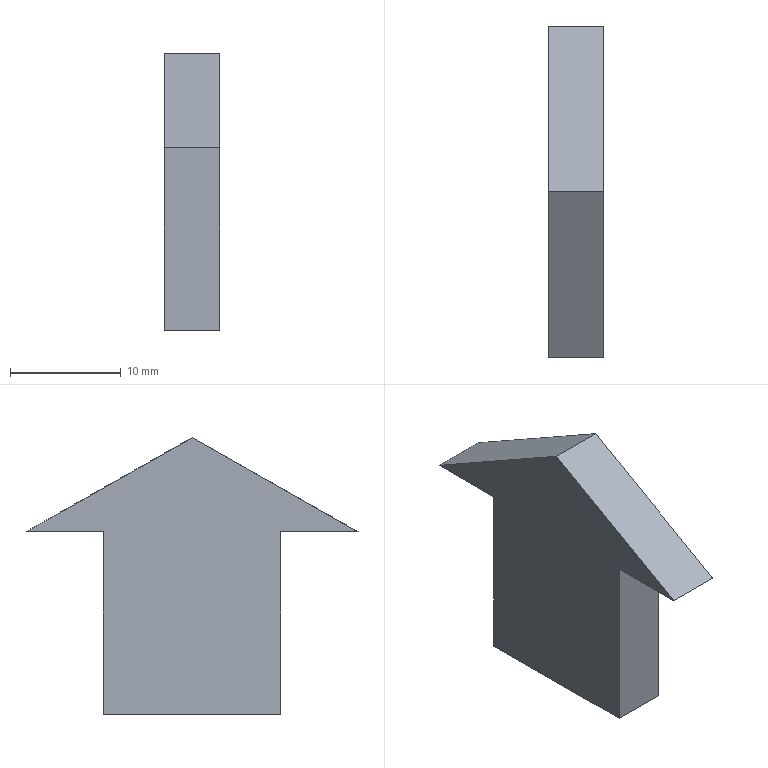Part | STEP file | 2_2_1-- | 1 solid | 9 faces | box 5 x 30 x 25 mm | volume 1957 mm3 | plane 9
STEP:
#1=CARTESIAN_POINT('',(0.,0.,0.));
#2=DIRECTION('',(0.,0.,1.));
#3=DIRECTION('',(1.,0.,0.));
#4=AXIS2_PLACEMENT_3D('',#1,#2,#3);
#5=CARTESIAN_POINT('',(-2.5,0.,50.));
#6=VERTEX_POINT('',#5);
#7=CARTESIAN_POINT('',(-2.5,-15.,41.5));
#8=VERTEX_POINT('',#7);
#9=CARTESIAN_POINT('',(-2.5,0.,50.));
#10=DIRECTION('',(0.,-0.87,-0.493));
#11=VECTOR('',#10,1.);
#12=LINE('',#9,#11);
#13=CARTESIAN_POINT('',(-2.5,0.,50.));
#14=DIRECTION('',(1.,0.,0.));
#15=DIRECTION('',(0.,0.,-1.));
#16=AXIS2_PLACEMENT_3D('',#13,#14,#15);
#17=PLANE('',#16);
#18=CARTESIAN_POINT('',(0.,0.));
#19=DIRECTION('',(0.493,-0.87));
#20=VECTOR('',#19,1.);
#21=LINE('',#18,#20);
#22=(GEOMETRIC_REPRESENTATION_CONTEXT(2)PARAMETRIC_REPRESENTATION_CONTEXT()REPRESENTATION_CONTEXT('',''));
#23=DEFINITIONAL_REPRESENTATION('',(#21),#22);
#24=PCURVE('',#17,#23);
#25=CARTESIAN_POINT('',(2.5,0.,50.));
#26=DIRECTION('',(0.,-0.493,0.87));
#27=DIRECTION('',(0.,-0.87,-0.493));
#28=AXIS2_PLACEMENT_3D('',#25,#26,#27);
#29=PLANE('',#28);
#30=CARTESIAN_POINT('',(0.,-5.));
#31=DIRECTION('',(1.,0.));
#32=VECTOR('',#31,1.);
#33=LINE('',#30,#32);
#34=(GEOMETRIC_REPRESENTATION_CONTEXT(2)PARAMETRIC_REPRESENTATION_CONTEXT()REPRESENTATION_CONTEXT('',''));
#35=DEFINITIONAL_REPRESENTATION('',(#33),#34);
#36=PCURVE('',#29,#35);
#37=SURFACE_CURVE('',#12,(#24,#36),.PCURVE_S1.);
#38=EDGE_CURVE('',#6,#8,#37,.T.);
#39=ORIENTED_EDGE('',*,*,#38,.F.);
#40=CARTESIAN_POINT('',(-2.5,15.,41.5));
#41=VERTEX_POINT('',#40);
#42=CARTESIAN_POINT('',(-2.5,15.,41.5));
#43=DIRECTION('',(0.,-0.87,0.493));
#44=VECTOR('',#43,1.);
#45=LINE('',#42,#44);
#46=CARTESIAN_POINT('',(8.5,15.));
#47=DIRECTION('',(-0.493,-0.87));
#48=VECTOR('',#47,1.);
#49=LINE('',#46,#48);
#50=(GEOMETRIC_REPRESENTATION_CONTEXT(2)PARAMETRIC_REPRESENTATION_CONTEXT()REPRESENTATION_CONTEXT('',''));
#51=DEFINITIONAL_REPRESENTATION('',(#49),#50);
#52=PCURVE('',#17,#51);
#53=CARTESIAN_POINT('',(2.5,15.,41.5));
#54=DIRECTION('',(0.,0.493,0.87));
#55=DIRECTION('',(0.,-0.87,0.493));
#56=AXIS2_PLACEMENT_3D('',#53,#54,#55);
#57=PLANE('',#56);
#58=CARTESIAN_POINT('',(0.,-5.));
#59=DIRECTION('',(1.,0.));
#60=VECTOR('',#59,1.);
#61=LINE('',#58,#60);
#62=(GEOMETRIC_REPRESENTATION_CONTEXT(2)PARAMETRIC_REPRESENTATION_CONTEXT()REPRESENTATION_CONTEXT('',''));
#63=DEFINITIONAL_REPRESENTATION('',(#61),#62);
#64=PCURVE('',#57,#63);
#65=SURFACE_CURVE('',#45,(#52,#64),.PCURVE_S1.);
#66=EDGE_CURVE('',#41,#6,#65,.T.);
#67=ORIENTED_EDGE('',*,*,#66,.F.);
#68=CARTESIAN_POINT('',(-2.5,8.,41.5));
#69=VERTEX_POINT('',#68);
#70=CARTESIAN_POINT('',(-2.5,0.,41.5));
#71=DIRECTION('',(0.,1.,0.));
#72=VECTOR('',#71,1.);
#73=LINE('',#70,#72);
#74=CARTESIAN_POINT('',(8.5,0.));
#75=DIRECTION('',(0.,1.));
#76=VECTOR('',#75,1.);
#77=LINE('',#74,#76);
#78=(GEOMETRIC_REPRESENTATION_CONTEXT(2)PARAMETRIC_REPRESENTATION_CONTEXT()REPRESENTATION_CONTEXT('',''));
#79=DEFINITIONAL_REPRESENTATION('',(#77),#78);
#80=PCURVE('',#17,#79);
#81=CARTESIAN_POINT('',(2.5,8.,41.5));
#82=DIRECTION('',(0.,0.,-1.));
#83=DIRECTION('',(-1.,0.,0.));
#84=AXIS2_PLACEMENT_3D('',#81,#82,#83);
#85=PLANE('',#84);
#86=CARTESIAN_POINT('',(5.,-8.));
#87=DIRECTION('',(0.,1.));
#88=VECTOR('',#87,1.);
#89=LINE('',#86,#88);
#90=(GEOMETRIC_REPRESENTATION_CONTEXT(2)PARAMETRIC_REPRESENTATION_CONTEXT()REPRESENTATION_CONTEXT('',''));
#91=DEFINITIONAL_REPRESENTATION('',(#89),#90);
#92=PCURVE('',#85,#91);
#93=SURFACE_CURVE('',#73,(#80,#92),.PCURVE_S1.);
#94=EDGE_CURVE('',#69,#41,#93,.T.);
#95=ORIENTED_EDGE('',*,*,#94,.F.);
#96=CARTESIAN_POINT('',(-2.5,8.,25.));
#97=VERTEX_POINT('',#96);
#98=CARTESIAN_POINT('',(-2.5,8.,50.));
#99=DIRECTION('',(0.,0.,1.));
#100=VECTOR('',#99,1.);
#101=LINE('',#98,#100);
#102=CARTESIAN_POINT('',(0.,8.));
#103=DIRECTION('',(-1.,0.));
#104=VECTOR('',#103,1.);
#105=LINE('',#102,#104);
#106=(GEOMETRIC_REPRESENTATION_CONTEXT(2)PARAMETRIC_REPRESENTATION_CONTEXT()REPRESENTATION_CONTEXT('',''));
#107=DEFINITIONAL_REPRESENTATION('',(#105),#106);
#108=PCURVE('',#17,#107);
#109=CARTESIAN_POINT('',(2.5,8.,25.));
#110=DIRECTION('',(0.,1.,0.));
#111=DIRECTION('',(0.,0.,1.));
#112=AXIS2_PLACEMENT_3D('',#109,#110,#111);
#113=PLANE('',#112);
#114=CARTESIAN_POINT('',(25.,-5.));
#115=DIRECTION('',(1.,0.));
#116=VECTOR('',#115,1.);
#117=LINE('',#114,#116);
#118=(GEOMETRIC_REPRESENTATION_CONTEXT(2)PARAMETRIC_REPRESENTATION_CONTEXT()REPRESENTATION_CONTEXT('',''));
#119=DEFINITIONAL_REPRESENTATION('',(#117),#118);
#120=PCURVE('',#113,#119);
#121=SURFACE_CURVE('',#101,(#108,#120),.PCURVE_S1.);
#122=EDGE_CURVE('',#97,#69,#121,.T.);
#123=ORIENTED_EDGE('',*,*,#122,.F.);
#124=CARTESIAN_POINT('',(-2.5,-8.,25.));
#125=VERTEX_POINT('',#124);
#126=CARTESIAN_POINT('',(-2.5,0.,25.));
#127=DIRECTION('',(0.,1.,0.));
#128=VECTOR('',#127,1.);
#129=LINE('',#126,#128);
#130=CARTESIAN_POINT('',(25.,0.));
#131=DIRECTION('',(0.,1.));
#132=VECTOR('',#131,1.);
#133=LINE('',#130,#132);
#134=(GEOMETRIC_REPRESENTATION_CONTEXT(2)PARAMETRIC_REPRESENTATION_CONTEXT()REPRESENTATION_CONTEXT('',''));
#135=DEFINITIONAL_REPRESENTATION('',(#133),#134);
#136=PCURVE('',#17,#135);
#137=CARTESIAN_POINT('',(2.5,-8.,25.));
#138=DIRECTION('',(0.,0.,-1.));
#139=DIRECTION('',(-1.,0.,0.));
#140=AXIS2_PLACEMENT_3D('',#137,#138,#139);
#141=PLANE('',#140);
#142=CARTESIAN_POINT('',(5.,8.));
#143=DIRECTION('',(0.,1.));
#144=VECTOR('',#143,1.);
#145=LINE('',#142,#144);
#146=(GEOMETRIC_REPRESENTATION_CONTEXT(2)PARAMETRIC_REPRESENTATION_CONTEXT()REPRESENTATION_CONTEXT('',''));
#147=DEFINITIONAL_REPRESENTATION('',(#145),#146);
#148=PCURVE('',#141,#147);
#149=SURFACE_CURVE('',#129,(#136,#148),.PCURVE_S1.);
#150=EDGE_CURVE('',#125,#97,#149,.T.);
#151=ORIENTED_EDGE('',*,*,#150,.F.);
#152=CARTESIAN_POINT('',(-2.5,-8.,41.5));
#153=VERTEX_POINT('',#152);
#154=CARTESIAN_POINT('',(-2.5,-8.,50.));
#155=DIRECTION('',(0.,0.,-1.));
#156=VECTOR('',#155,1.);
#157=LINE('',#154,#156);
#158=CARTESIAN_POINT('',(0.,-8.));
#159=DIRECTION('',(1.,0.));
#160=VECTOR('',#159,1.);
#161=LINE('',#158,#160);
#162=(GEOMETRIC_REPRESENTATION_CONTEXT(2)PARAMETRIC_REPRESENTATION_CONTEXT()REPRESENTATION_CONTEXT('',''));
#163=DEFINITIONAL_REPRESENTATION('',(#161),#162);
#164=PCURVE('',#17,#163);
#165=CARTESIAN_POINT('',(2.5,-8.,41.5));
#166=DIRECTION('',(0.,-1.,0.));
#167=DIRECTION('',(0.,0.,-1.));
#168=AXIS2_PLACEMENT_3D('',#165,#166,#167);
#169=PLANE('',#168);
#170=CARTESIAN_POINT('',(-8.5,-5.));
#171=DIRECTION('',(1.,0.));
#172=VECTOR('',#171,1.);
#173=LINE('',#170,#172);
#174=(GEOMETRIC_REPRESENTATION_CONTEXT(2)PARAMETRIC_REPRESENTATION_CONTEXT()REPRESENTATION_CONTEXT('',''));
#175=DEFINITIONAL_REPRESENTATION('',(#173),#174);
#176=PCURVE('',#169,#175);
#177=SURFACE_CURVE('',#157,(#164,#176),.PCURVE_S1.);
#178=EDGE_CURVE('',#153,#125,#177,.T.);
#179=ORIENTED_EDGE('',*,*,#178,.F.);
#180=CARTESIAN_POINT('',(-2.5,0.,41.5));
#181=DIRECTION('',(0.,1.,0.));
#182=VECTOR('',#181,1.);
#183=LINE('',#180,#182);
#184=CARTESIAN_POINT('',(8.5,0.));
#185=DIRECTION('',(0.,1.));
#186=VECTOR('',#185,1.);
#187=LINE('',#184,#186);
#188=(GEOMETRIC_REPRESENTATION_CONTEXT(2)PARAMETRIC_REPRESENTATION_CONTEXT()REPRESENTATION_CONTEXT('',''));
#189=DEFINITIONAL_REPRESENTATION('',(#187),#188);
#190=PCURVE('',#17,#189);
#191=CARTESIAN_POINT('',(2.5,-15.,41.5));
#192=DIRECTION('',(0.,0.,-1.));
#193=DIRECTION('',(-1.,0.,0.));
#194=AXIS2_PLACEMENT_3D('',#191,#192,#193);
#195=PLANE('',#194);
#196=CARTESIAN_POINT('',(5.,15.));
#197=DIRECTION('',(0.,1.));
#198=VECTOR('',#197,1.);
#199=LINE('',#196,#198);
#200=(GEOMETRIC_REPRESENTATION_CONTEXT(2)PARAMETRIC_REPRESENTATION_CONTEXT()REPRESENTATION_CONTEXT('',''));
#201=DEFINITIONAL_REPRESENTATION('',(#199),#200);
#202=PCURVE('',#195,#201);
#203=SURFACE_CURVE('',#183,(#190,#202),.PCURVE_S1.);
#204=EDGE_CURVE('',#8,#153,#203,.T.);
#205=ORIENTED_EDGE('',*,*,#204,.F.);
#206=EDGE_LOOP('',(#39,#67,#95,#123,#151,#179,#205));
#207=FACE_BOUND('',#206,.T.);
#208=ADVANCED_FACE('',(#207),#17,.F.);
#209=CARTESIAN_POINT('',(2.5,-8.,41.5));
#210=VERTEX_POINT('',#209);
#211=CARTESIAN_POINT('',(2.5,-15.,41.5));
#212=VERTEX_POINT('',#211);
#213=CARTESIAN_POINT('',(2.5,-15.,41.5));
#214=DIRECTION('',(0.,-1.,0.));
#215=VECTOR('',#214,1.);
#216=LINE('',#213,#215);
#217=CARTESIAN_POINT('',(0.,0.));
#218=DIRECTION('',(0.,-1.));
#219=VECTOR('',#218,1.);
#220=LINE('',#217,#219);
#221=(GEOMETRIC_REPRESENTATION_CONTEXT(2)PARAMETRIC_REPRESENTATION_CONTEXT()REPRESENTATION_CONTEXT('',''));
#222=DEFINITIONAL_REPRESENTATION('',(#220),#221);
#223=PCURVE('',#195,#222);
#224=CARTESIAN_POINT('',(2.5,0.,50.));
#225=DIRECTION('',(1.,0.,0.));
#226=DIRECTION('',(0.,0.,-1.));
#227=AXIS2_PLACEMENT_3D('',#224,#225,#226);
#228=PLANE('',#227);
#229=CARTESIAN_POINT('',(8.5,-15.));
#230=DIRECTION('',(0.,-1.));
#231=VECTOR('',#230,1.);
#232=LINE('',#229,#231);
#233=(GEOMETRIC_REPRESENTATION_CONTEXT(2)PARAMETRIC_REPRESENTATION_CONTEXT()REPRESENTATION_CONTEXT('',''));
#234=DEFINITIONAL_REPRESENTATION('',(#232),#233);
#235=PCURVE('',#228,#234);
#236=SURFACE_CURVE('',#216,(#223,#235),.PCURVE_S1.);
#237=EDGE_CURVE('',#210,#212,#236,.T.);
#238=ORIENTED_EDGE('',*,*,#237,.T.);
#239=CARTESIAN_POINT('',(2.5,-15.,41.5));
#240=DIRECTION('',(-1.,0.,0.));
#241=VECTOR('',#240,1.);
#242=LINE('',#239,#241);
#243=CARTESIAN_POINT('',(0.,0.));
#244=DIRECTION('',(1.,0.));
#245=VECTOR('',#244,1.);
#246=LINE('',#243,#245);
#247=(GEOMETRIC_REPRESENTATION_CONTEXT(2)PARAMETRIC_REPRESENTATION_CONTEXT()REPRESENTATION_CONTEXT('',''));
#248=DEFINITIONAL_REPRESENTATION('',(#246),#247);
#249=PCURVE('',#195,#248);
#250=CARTESIAN_POINT('',(17.241,0.));
#251=DIRECTION('',(0.,-1.));
#252=VECTOR('',#251,1.);
#253=LINE('',#250,#252);
#254=(GEOMETRIC_REPRESENTATION_CONTEXT(2)PARAMETRIC_REPRESENTATION_CONTEXT()REPRESENTATION_CONTEXT('',''));
#255=DEFINITIONAL_REPRESENTATION('',(#253),#254);
#256=PCURVE('',#29,#255);
#257=SURFACE_CURVE('',#242,(#249,#256),.PCURVE_S1.);
#258=EDGE_CURVE('',#212,#8,#257,.T.);
#259=ORIENTED_EDGE('',*,*,#258,.T.);
#260=ORIENTED_EDGE('',*,*,#204,.T.);
#261=CARTESIAN_POINT('',(2.5,-8.,41.5));
#262=DIRECTION('',(1.,0.,0.));
#263=VECTOR('',#262,1.);
#264=LINE('',#261,#263);
#265=CARTESIAN_POINT('',(0.,7.));
#266=DIRECTION('',(-1.,0.));
#267=VECTOR('',#266,1.);
#268=LINE('',#265,#267);
#269=(GEOMETRIC_REPRESENTATION_CONTEXT(2)PARAMETRIC_REPRESENTATION_CONTEXT()REPRESENTATION_CONTEXT('',''));
#270=DEFINITIONAL_REPRESENTATION('',(#268),#269);
#271=PCURVE('',#195,#270);
#272=CARTESIAN_POINT('',(0.,0.));
#273=DIRECTION('',(0.,1.));
#274=VECTOR('',#273,1.);
#275=LINE('',#272,#274);
#276=(GEOMETRIC_REPRESENTATION_CONTEXT(2)PARAMETRIC_REPRESENTATION_CONTEXT()REPRESENTATION_CONTEXT('',''));
#277=DEFINITIONAL_REPRESENTATION('',(#275),#276);
#278=PCURVE('',#169,#277);
#279=SURFACE_CURVE('',#264,(#271,#278),.PCURVE_S1.);
#280=EDGE_CURVE('',#153,#210,#279,.T.);
#281=ORIENTED_EDGE('',*,*,#280,.T.);
#282=EDGE_LOOP('',(#238,#259,#260,#281));
#283=FACE_BOUND('',#282,.T.);
#284=ADVANCED_FACE('',(#283),#195,.T.);
#285=CARTESIAN_POINT('',(2.5,0.,50.));
#286=VERTEX_POINT('',#285);
#287=CARTESIAN_POINT('',(2.5,0.,50.));
#288=DIRECTION('',(0.,0.87,0.493));
#289=VECTOR('',#288,1.);
#290=LINE('',#287,#289);
#291=CARTESIAN_POINT('',(0.,0.));
#292=DIRECTION('',(-1.,0.));
#293=VECTOR('',#292,1.);
#294=LINE('',#291,#293);
#295=(GEOMETRIC_REPRESENTATION_CONTEXT(2)PARAMETRIC_REPRESENTATION_CONTEXT()REPRESENTATION_CONTEXT('',''));
#296=DEFINITIONAL_REPRESENTATION('',(#294),#295);
#297=PCURVE('',#29,#296);
#298=CARTESIAN_POINT('',(0.,0.));
#299=DIRECTION('',(-0.493,0.87));
#300=VECTOR('',#299,1.);
#301=LINE('',#298,#300);
#302=(GEOMETRIC_REPRESENTATION_CONTEXT(2)PARAMETRIC_REPRESENTATION_CONTEXT()REPRESENTATION_CONTEXT('',''));
#303=DEFINITIONAL_REPRESENTATION('',(#301),#302);
#304=PCURVE('',#228,#303);
#305=SURFACE_CURVE('',#290,(#297,#304),.PCURVE_S1.);
#306=EDGE_CURVE('',#212,#286,#305,.T.);
#307=ORIENTED_EDGE('',*,*,#306,.T.);
#308=CARTESIAN_POINT('',(2.5,0.,50.));
#309=DIRECTION('',(-1.,0.,0.));
#310=VECTOR('',#309,1.);
#311=LINE('',#308,#310);
#312=CARTESIAN_POINT('',(0.,0.));
#313=DIRECTION('',(0.,-1.));
#314=VECTOR('',#313,1.);
#315=LINE('',#312,#314);
#316=(GEOMETRIC_REPRESENTATION_CONTEXT(2)PARAMETRIC_REPRESENTATION_CONTEXT()REPRESENTATION_CONTEXT('',''));
#317=DEFINITIONAL_REPRESENTATION('',(#315),#316);
#318=PCURVE('',#29,#317);
#319=CARTESIAN_POINT('',(17.241,0.));
#320=DIRECTION('',(0.,-1.));
#321=VECTOR('',#320,1.);
#322=LINE('',#319,#321);
#323=(GEOMETRIC_REPRESENTATION_CONTEXT(2)PARAMETRIC_REPRESENTATION_CONTEXT()REPRESENTATION_CONTEXT('',''));
#324=DEFINITIONAL_REPRESENTATION('',(#322),#323);
#325=PCURVE('',#57,#324);
#326=SURFACE_CURVE('',#311,(#318,#325),.PCURVE_S1.);
#327=EDGE_CURVE('',#286,#6,#326,.T.);
#328=ORIENTED_EDGE('',*,*,#327,.T.);
#329=ORIENTED_EDGE('',*,*,#38,.T.);
#330=ORIENTED_EDGE('',*,*,#258,.F.);
#331=EDGE_LOOP('',(#307,#328,#329,#330));
#332=FACE_BOUND('',#331,.T.);
#333=ADVANCED_FACE('',(#332),#29,.T.);
#334=CARTESIAN_POINT('',(2.5,15.,41.5));
#335=VERTEX_POINT('',#334);
#336=CARTESIAN_POINT('',(2.5,15.,41.5));
#337=DIRECTION('',(0.,0.87,-0.493));
#338=VECTOR('',#337,1.);
#339=LINE('',#336,#338);
#340=CARTESIAN_POINT('',(0.,0.));
#341=DIRECTION('',(-1.,0.));
#342=VECTOR('',#341,1.);
#343=LINE('',#340,#342);
#344=(GEOMETRIC_REPRESENTATION_CONTEXT(2)PARAMETRIC_REPRESENTATION_CONTEXT()REPRESENTATION_CONTEXT('',''));
#345=DEFINITIONAL_REPRESENTATION('',(#343),#344);
#346=PCURVE('',#57,#345);
#347=CARTESIAN_POINT('',(8.5,15.));
#348=DIRECTION('',(0.493,0.87));
#349=VECTOR('',#348,1.);
#350=LINE('',#347,#349);
#351=(GEOMETRIC_REPRESENTATION_CONTEXT(2)PARAMETRIC_REPRESENTATION_CONTEXT()REPRESENTATION_CONTEXT('',''));
#352=DEFINITIONAL_REPRESENTATION('',(#350),#351);
#353=PCURVE('',#228,#352);
#354=SURFACE_CURVE('',#339,(#346,#353),.PCURVE_S1.);
#355=EDGE_CURVE('',#286,#335,#354,.T.);
#356=ORIENTED_EDGE('',*,*,#355,.T.);
#357=CARTESIAN_POINT('',(2.5,15.,41.5));
#358=DIRECTION('',(-1.,0.,0.));
#359=VECTOR('',#358,1.);
#360=LINE('',#357,#359);
#361=CARTESIAN_POINT('',(0.,0.));
#362=DIRECTION('',(0.,-1.));
#363=VECTOR('',#362,1.);
#364=LINE('',#361,#363);
#365=(GEOMETRIC_REPRESENTATION_CONTEXT(2)PARAMETRIC_REPRESENTATION_CONTEXT()REPRESENTATION_CONTEXT('',''));
#366=DEFINITIONAL_REPRESENTATION('',(#364),#365);
#367=PCURVE('',#57,#366);
#368=CARTESIAN_POINT('',(0.,7.));
#369=DIRECTION('',(1.,0.));
#370=VECTOR('',#369,1.);
#371=LINE('',#368,#370);
#372=(GEOMETRIC_REPRESENTATION_CONTEXT(2)PARAMETRIC_REPRESENTATION_CONTEXT()REPRESENTATION_CONTEXT('',''));
#373=DEFINITIONAL_REPRESENTATION('',(#371),#372);
#374=PCURVE('',#85,#373);
#375=SURFACE_CURVE('',#360,(#367,#374),.PCURVE_S1.);
#376=EDGE_CURVE('',#335,#41,#375,.T.);
#377=ORIENTED_EDGE('',*,*,#376,.T.);
#378=ORIENTED_EDGE('',*,*,#66,.T.);
#379=ORIENTED_EDGE('',*,*,#327,.F.);
#380=EDGE_LOOP('',(#356,#377,#378,#379));
#381=FACE_BOUND('',#380,.T.);
#382=ADVANCED_FACE('',(#381),#57,.T.);
#383=CARTESIAN_POINT('',(2.5,8.,41.5));
#384=VERTEX_POINT('',#383);
#385=CARTESIAN_POINT('',(2.5,8.,41.5));
#386=DIRECTION('',(0.,-1.,0.));
#387=VECTOR('',#386,1.);
#388=LINE('',#385,#387);
#389=CARTESIAN_POINT('',(0.,0.));
#390=DIRECTION('',(0.,-1.));
#391=VECTOR('',#390,1.);
#392=LINE('',#389,#391);
#393=(GEOMETRIC_REPRESENTATION_CONTEXT(2)PARAMETRIC_REPRESENTATION_CONTEXT()REPRESENTATION_CONTEXT('',''));
#394=DEFINITIONAL_REPRESENTATION('',(#392),#393);
#395=PCURVE('',#85,#394);
#396=CARTESIAN_POINT('',(8.5,8.));
#397=DIRECTION('',(0.,-1.));
#398=VECTOR('',#397,1.);
#399=LINE('',#396,#398);
#400=(GEOMETRIC_REPRESENTATION_CONTEXT(2)PARAMETRIC_REPRESENTATION_CONTEXT()REPRESENTATION_CONTEXT('',''));
#401=DEFINITIONAL_REPRESENTATION('',(#399),#400);
#402=PCURVE('',#228,#401);
#403=SURFACE_CURVE('',#388,(#395,#402),.PCURVE_S1.);
#404=EDGE_CURVE('',#335,#384,#403,.T.);
#405=ORIENTED_EDGE('',*,*,#404,.T.);
#406=CARTESIAN_POINT('',(2.5,8.,41.5));
#407=DIRECTION('',(-1.,0.,0.));
#408=VECTOR('',#407,1.);
#409=LINE('',#406,#408);
#410=CARTESIAN_POINT('',(0.,0.));
#411=DIRECTION('',(1.,0.));
#412=VECTOR('',#411,1.);
#413=LINE('',#410,#412);
#414=(GEOMETRIC_REPRESENTATION_CONTEXT(2)PARAMETRIC_REPRESENTATION_CONTEXT()REPRESENTATION_CONTEXT('',''));
#415=DEFINITIONAL_REPRESENTATION('',(#413),#414);
#416=PCURVE('',#85,#415);
#417=CARTESIAN_POINT('',(16.5,0.));
#418=DIRECTION('',(0.,-1.));
#419=VECTOR('',#418,1.);
#420=LINE('',#417,#419);
#421=(GEOMETRIC_REPRESENTATION_CONTEXT(2)PARAMETRIC_REPRESENTATION_CONTEXT()REPRESENTATION_CONTEXT('',''));
#422=DEFINITIONAL_REPRESENTATION('',(#420),#421);
#423=PCURVE('',#113,#422);
#424=SURFACE_CURVE('',#409,(#416,#423),.PCURVE_S1.);
#425=EDGE_CURVE('',#384,#69,#424,.T.);
#426=ORIENTED_EDGE('',*,*,#425,.T.);
#427=ORIENTED_EDGE('',*,*,#94,.T.);
#428=ORIENTED_EDGE('',*,*,#376,.F.);
#429=EDGE_LOOP('',(#405,#426,#427,#428));
#430=FACE_BOUND('',#429,.T.);
#431=ADVANCED_FACE('',(#430),#85,.T.);
#432=CARTESIAN_POINT('',(2.5,8.,25.));
#433=VERTEX_POINT('',#432);
#434=CARTESIAN_POINT('',(2.5,8.,25.));
#435=DIRECTION('',(0.,0.,-1.));
#436=VECTOR('',#435,1.);
#437=LINE('',#434,#436);
#438=CARTESIAN_POINT('',(0.,0.));
#439=DIRECTION('',(-1.,0.));
#440=VECTOR('',#439,1.);
#441=LINE('',#438,#440);
#442=(GEOMETRIC_REPRESENTATION_CONTEXT(2)PARAMETRIC_REPRESENTATION_CONTEXT()REPRESENTATION_CONTEXT('',''));
#443=DEFINITIONAL_REPRESENTATION('',(#441),#442);
#444=PCURVE('',#113,#443);
#445=CARTESIAN_POINT('',(25.,8.));
#446=DIRECTION('',(1.,0.));
#447=VECTOR('',#446,1.);
#448=LINE('',#445,#447);
#449=(GEOMETRIC_REPRESENTATION_CONTEXT(2)PARAMETRIC_REPRESENTATION_CONTEXT()REPRESENTATION_CONTEXT('',''));
#450=DEFINITIONAL_REPRESENTATION('',(#448),#449);
#451=PCURVE('',#228,#450);
#452=SURFACE_CURVE('',#437,(#444,#451),.PCURVE_S1.);
#453=EDGE_CURVE('',#384,#433,#452,.T.);
#454=ORIENTED_EDGE('',*,*,#453,.T.);
#455=CARTESIAN_POINT('',(2.5,8.,25.));
#456=DIRECTION('',(-1.,0.,0.));
#457=VECTOR('',#456,1.);
#458=LINE('',#455,#457);
#459=CARTESIAN_POINT('',(0.,0.));
#460=DIRECTION('',(0.,-1.));
#461=VECTOR('',#460,1.);
#462=LINE('',#459,#461);
#463=(GEOMETRIC_REPRESENTATION_CONTEXT(2)PARAMETRIC_REPRESENTATION_CONTEXT()REPRESENTATION_CONTEXT('',''));
#464=DEFINITIONAL_REPRESENTATION('',(#462),#463);
#465=PCURVE('',#113,#464);
#466=CARTESIAN_POINT('',(0.,16.));
#467=DIRECTION('',(1.,0.));
#468=VECTOR('',#467,1.);
#469=LINE('',#466,#468);
#470=(GEOMETRIC_REPRESENTATION_CONTEXT(2)PARAMETRIC_REPRESENTATION_CONTEXT()REPRESENTATION_CONTEXT('',''));
#471=DEFINITIONAL_REPRESENTATION('',(#469),#470);
#472=PCURVE('',#141,#471);
#473=SURFACE_CURVE('',#458,(#465,#472),.PCURVE_S1.);
#474=EDGE_CURVE('',#433,#97,#473,.T.);
#475=ORIENTED_EDGE('',*,*,#474,.T.);
#476=ORIENTED_EDGE('',*,*,#122,.T.);
#477=ORIENTED_EDGE('',*,*,#425,.F.);
#478=EDGE_LOOP('',(#454,#475,#476,#477));
#479=FACE_BOUND('',#478,.T.);
#480=ADVANCED_FACE('',(#479),#113,.T.);
#481=CARTESIAN_POINT('',(2.5,-8.,25.));
#482=VERTEX_POINT('',#481);
#483=CARTESIAN_POINT('',(2.5,-8.,25.));
#484=DIRECTION('',(0.,-1.,0.));
#485=VECTOR('',#484,1.);
#486=LINE('',#483,#485);
#487=CARTESIAN_POINT('',(0.,0.));
#488=DIRECTION('',(0.,-1.));
#489=VECTOR('',#488,1.);
#490=LINE('',#487,#489);
#491=(GEOMETRIC_REPRESENTATION_CONTEXT(2)PARAMETRIC_REPRESENTATION_CONTEXT()REPRESENTATION_CONTEXT('',''));
#492=DEFINITIONAL_REPRESENTATION('',(#490),#491);
#493=PCURVE('',#141,#492);
#494=CARTESIAN_POINT('',(25.,-8.));
#495=DIRECTION('',(0.,-1.));
#496=VECTOR('',#495,1.);
#497=LINE('',#494,#496);
#498=(GEOMETRIC_REPRESENTATION_CONTEXT(2)PARAMETRIC_REPRESENTATION_CONTEXT()REPRESENTATION_CONTEXT('',''));
#499=DEFINITIONAL_REPRESENTATION('',(#497),#498);
#500=PCURVE('',#228,#499);
#501=SURFACE_CURVE('',#486,(#493,#500),.PCURVE_S1.);
#502=EDGE_CURVE('',#433,#482,#501,.T.);
#503=ORIENTED_EDGE('',*,*,#502,.T.);
#504=CARTESIAN_POINT('',(2.5,-8.,25.));
#505=DIRECTION('',(-1.,0.,0.));
#506=VECTOR('',#505,1.);
#507=LINE('',#504,#506);
#508=CARTESIAN_POINT('',(0.,0.));
#509=DIRECTION('',(1.,0.));
#510=VECTOR('',#509,1.);
#511=LINE('',#508,#510);
#512=(GEOMETRIC_REPRESENTATION_CONTEXT(2)PARAMETRIC_REPRESENTATION_CONTEXT()REPRESENTATION_CONTEXT('',''));
#513=DEFINITIONAL_REPRESENTATION('',(#511),#512);
#514=PCURVE('',#141,#513);
#515=CARTESIAN_POINT('',(16.5,0.));
#516=DIRECTION('',(0.,-1.));
#517=VECTOR('',#516,1.);
#518=LINE('',#515,#517);
#519=(GEOMETRIC_REPRESENTATION_CONTEXT(2)PARAMETRIC_REPRESENTATION_CONTEXT()REPRESENTATION_CONTEXT('',''));
#520=DEFINITIONAL_REPRESENTATION('',(#518),#519);
#521=PCURVE('',#169,#520);
#522=SURFACE_CURVE('',#507,(#514,#521),.PCURVE_S1.);
#523=EDGE_CURVE('',#482,#125,#522,.T.);
#524=ORIENTED_EDGE('',*,*,#523,.T.);
#525=ORIENTED_EDGE('',*,*,#150,.T.);
#526=ORIENTED_EDGE('',*,*,#474,.F.);
#527=EDGE_LOOP('',(#503,#524,#525,#526));
#528=FACE_BOUND('',#527,.T.);
#529=ADVANCED_FACE('',(#528),#141,.T.);
#530=CARTESIAN_POINT('',(2.5,-8.,41.5));
#531=DIRECTION('',(0.,0.,1.));
#532=VECTOR('',#531,1.);
#533=LINE('',#530,#532);
#534=CARTESIAN_POINT('',(0.,0.));
#535=DIRECTION('',(-1.,0.));
#536=VECTOR('',#535,1.);
#537=LINE('',#534,#536);
#538=(GEOMETRIC_REPRESENTATION_CONTEXT(2)PARAMETRIC_REPRESENTATION_CONTEXT()REPRESENTATION_CONTEXT('',''));
#539=DEFINITIONAL_REPRESENTATION('',(#537),#538);
#540=PCURVE('',#169,#539);
#541=CARTESIAN_POINT('',(8.5,-8.));
#542=DIRECTION('',(-1.,0.));
#543=VECTOR('',#542,1.);
#544=LINE('',#541,#543);
#545=(GEOMETRIC_REPRESENTATION_CONTEXT(2)PARAMETRIC_REPRESENTATION_CONTEXT()REPRESENTATION_CONTEXT('',''));
#546=DEFINITIONAL_REPRESENTATION('',(#544),#545);
#547=PCURVE('',#228,#546);
#548=SURFACE_CURVE('',#533,(#540,#547),.PCURVE_S1.);
#549=EDGE_CURVE('',#482,#210,#548,.T.);
#550=ORIENTED_EDGE('',*,*,#549,.T.);
#551=ORIENTED_EDGE('',*,*,#280,.F.);
#552=ORIENTED_EDGE('',*,*,#178,.T.);
#553=ORIENTED_EDGE('',*,*,#523,.F.);
#554=EDGE_LOOP('',(#550,#551,#552,#553));
#555=FACE_BOUND('',#554,.T.);
#556=ADVANCED_FACE('',(#555),#169,.T.);
#557=ORIENTED_EDGE('',*,*,#404,.F.);
#558=ORIENTED_EDGE('',*,*,#355,.F.);
#559=ORIENTED_EDGE('',*,*,#306,.F.);
#560=ORIENTED_EDGE('',*,*,#237,.F.);
#561=ORIENTED_EDGE('',*,*,#549,.F.);
#562=ORIENTED_EDGE('',*,*,#502,.F.);
#563=ORIENTED_EDGE('',*,*,#453,.F.);
#564=EDGE_LOOP('',(#557,#558,#559,#560,#561,#562,#563));
#565=FACE_BOUND('',#564,.T.);
#566=ADVANCED_FACE('',(#565),#228,.T.);
#567=CLOSED_SHELL('',(#208,#284,#333,#382,#431,#480,#529,#556,#566));
#568=MANIFOLD_SOLID_BREP('',#567);
#569=(LENGTH_UNIT()NAMED_UNIT(*)SI_UNIT(.MILLI.,.METRE.));
#570=UNCERTAINTY_MEASURE_WITH_UNIT(LENGTH_MEASURE(0.0000001),#569,'','');
#571=(NAMED_UNIT(*)PLANE_ANGLE_UNIT()SI_UNIT($,.RADIAN.));
#572=(NAMED_UNIT(*)SI_UNIT($,.STERADIAN.)SOLID_ANGLE_UNIT());
#573=(GEOMETRIC_REPRESENTATION_CONTEXT(3)GLOBAL_UNCERTAINTY_ASSIGNED_CONTEXT((#570))GLOBAL_UNIT_ASSIGNED_CONTEXT((#569,#571,#572))REPRESENTATION_CONTEXT('',''));
#574=ADVANCED_BREP_SHAPE_REPRESENTATION('',(#4,#568),#573);